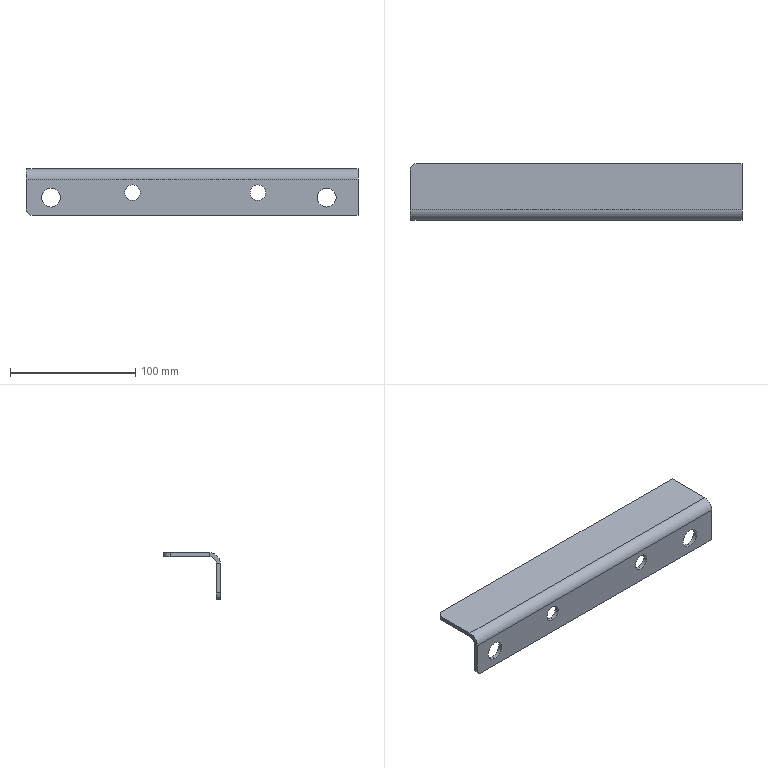Part | SolidWorks | features Fillet 1, FlatPattern 1, ICE 1, SMBaseFlange 1, SheetMetal 1 | 1 solid | 24 faces | box 265 x 45 x 37 mm | volume 62470 mm3 | cylinder 12 | plane 12 | commonest cylinder face diameters 12.5 x4 15 x4 10 x3 16.4 x1
STEP:
#1=CARTESIAN_POINT('',(-112.5,0.,-30.5));
#2=VERTEX_POINT('',#1);
#3=CARTESIAN_POINT('',(-112.5,0.,-15.5));
#4=VERTEX_POINT('',#3);
#5=CARTESIAN_POINT('',(-112.5,0.,-23.));
#6=DIRECTION('',(0.,1.,0.));
#7=DIRECTION('',(0.,0.,1.));
#8=AXIS2_PLACEMENT_3D('',#5,#6,#7);
#9=CIRCLE('',#8,7.5);
#10=EDGE_CURVE('',#2,#4,#9,.T.);
#11=ORIENTED_EDGE('',*,*,#10,.F.);
#12=CARTESIAN_POINT('',(-112.5,3.2,-30.5));
#13=VERTEX_POINT('',#12);
#14=CARTESIAN_POINT('',(-112.5,0.,-30.5));
#15=DIRECTION('',(0.,1.,0.));
#16=VECTOR('',#15,1000.);
#17=LINE('',#14,#16);
#18=EDGE_CURVE('',#2,#13,#17,.T.);
#19=ORIENTED_EDGE('',*,*,#18,.T.);
#20=CARTESIAN_POINT('',(-112.5,3.2,-15.5));
#21=VERTEX_POINT('',#20);
#22=CARTESIAN_POINT('',(-112.5,3.2,-23.));
#23=DIRECTION('',(0.,1.,0.));
#24=DIRECTION('',(0.,0.,1.));
#25=AXIS2_PLACEMENT_3D('',#22,#23,#24);
#26=CIRCLE('',#25,7.5);
#27=EDGE_CURVE('',#13,#21,#26,.T.);
#28=ORIENTED_EDGE('',*,*,#27,.T.);
#29=CARTESIAN_POINT('',(-112.5,0.,-15.5));
#30=DIRECTION('',(0.,1.,0.));
#31=VECTOR('',#30,1000.);
#32=LINE('',#29,#31);
#33=EDGE_CURVE('',#4,#21,#32,.T.);
#34=ORIENTED_EDGE('',*,*,#33,.F.);
#35=EDGE_LOOP('',(#11,#19,#28,#34));
#36=FACE_OUTER_BOUND('',#35,.T.);
#37=CARTESIAN_POINT('',(-112.5,0.,-23.));
#38=DIRECTION('',(0.,1.,0.));
#39=DIRECTION('',(0.,0.,1.));
#40=AXIS2_PLACEMENT_3D('',#37,#38,#39);
#41=CYLINDRICAL_SURFACE('',#40,7.5);
#42=ADVANCED_FACE('',(#36),#41,.F.);
#43=CARTESIAN_POINT('',(107.5,0.,-30.5));
#44=VERTEX_POINT('',#43);
#45=CARTESIAN_POINT('',(107.5,0.,-15.5));
#46=VERTEX_POINT('',#45);
#47=CARTESIAN_POINT('',(107.5,0.,-23.));
#48=DIRECTION('',(0.,1.,0.));
#49=DIRECTION('',(0.,0.,1.));
#50=AXIS2_PLACEMENT_3D('',#47,#48,#49);
#51=CIRCLE('',#50,7.5);
#52=EDGE_CURVE('',#44,#46,#51,.T.);
#53=ORIENTED_EDGE('',*,*,#52,.F.);
#54=CARTESIAN_POINT('',(107.5,3.2,-30.5));
#55=VERTEX_POINT('',#54);
#56=CARTESIAN_POINT('',(107.5,0.,-30.5));
#57=DIRECTION('',(0.,1.,0.));
#58=VECTOR('',#57,1000.);
#59=LINE('',#56,#58);
#60=EDGE_CURVE('',#44,#55,#59,.T.);
#61=ORIENTED_EDGE('',*,*,#60,.T.);
#62=CARTESIAN_POINT('',(107.5,3.2,-15.5));
#63=VERTEX_POINT('',#62);
#64=CARTESIAN_POINT('',(107.5,3.2,-23.));
#65=DIRECTION('',(0.,1.,0.));
#66=DIRECTION('',(0.,0.,1.));
#67=AXIS2_PLACEMENT_3D('',#64,#65,#66);
#68=CIRCLE('',#67,7.5);
#69=EDGE_CURVE('',#55,#63,#68,.T.);
#70=ORIENTED_EDGE('',*,*,#69,.T.);
#71=CARTESIAN_POINT('',(107.5,0.,-15.5));
#72=DIRECTION('',(0.,1.,0.));
#73=VECTOR('',#72,1000.);
#74=LINE('',#71,#73);
#75=EDGE_CURVE('',#46,#63,#74,.T.);
#76=ORIENTED_EDGE('',*,*,#75,.F.);
#77=EDGE_LOOP('',(#53,#61,#70,#76));
#78=FACE_OUTER_BOUND('',#77,.T.);
#79=CARTESIAN_POINT('',(107.5,0.,-23.));
#80=DIRECTION('',(0.,1.,0.));
#81=DIRECTION('',(0.,0.,1.));
#82=AXIS2_PLACEMENT_3D('',#79,#80,#81);
#83=CYLINDRICAL_SURFACE('',#82,7.5);
#84=ADVANCED_FACE('',(#78),#83,.F.);
#85=CARTESIAN_POINT('',(52.5,0.,-25.25));
#86=VERTEX_POINT('',#85);
#87=CARTESIAN_POINT('',(52.5,0.,-12.75));
#88=VERTEX_POINT('',#87);
#89=CARTESIAN_POINT('',(52.5,0.,-19.));
#90=DIRECTION('',(0.,1.,0.));
#91=DIRECTION('',(0.,0.,1.));
#92=AXIS2_PLACEMENT_3D('',#89,#90,#91);
#93=CIRCLE('',#92,6.25);
#94=EDGE_CURVE('',#86,#88,#93,.T.);
#95=ORIENTED_EDGE('',*,*,#94,.F.);
#96=CARTESIAN_POINT('',(52.5,3.2,-25.25));
#97=VERTEX_POINT('',#96);
#98=CARTESIAN_POINT('',(52.5,0.,-25.25));
#99=DIRECTION('',(0.,1.,0.));
#100=VECTOR('',#99,1000.);
#101=LINE('',#98,#100);
#102=EDGE_CURVE('',#86,#97,#101,.T.);
#103=ORIENTED_EDGE('',*,*,#102,.T.);
#104=CARTESIAN_POINT('',(52.5,3.2,-12.75));
#105=VERTEX_POINT('',#104);
#106=CARTESIAN_POINT('',(52.5,3.2,-19.));
#107=DIRECTION('',(0.,1.,0.));
#108=DIRECTION('',(0.,0.,1.));
#109=AXIS2_PLACEMENT_3D('',#106,#107,#108);
#110=CIRCLE('',#109,6.25);
#111=EDGE_CURVE('',#97,#105,#110,.T.);
#112=ORIENTED_EDGE('',*,*,#111,.T.);
#113=CARTESIAN_POINT('',(52.5,0.,-12.75));
#114=DIRECTION('',(0.,1.,0.));
#115=VECTOR('',#114,1000.);
#116=LINE('',#113,#115);
#117=EDGE_CURVE('',#88,#105,#116,.T.);
#118=ORIENTED_EDGE('',*,*,#117,.F.);
#119=EDGE_LOOP('',(#95,#103,#112,#118));
#120=FACE_OUTER_BOUND('',#119,.T.);
#121=CARTESIAN_POINT('',(52.5,0.,-19.));
#122=DIRECTION('',(0.,1.,0.));
#123=DIRECTION('',(0.,0.,1.));
#124=AXIS2_PLACEMENT_3D('',#121,#122,#123);
#125=CYLINDRICAL_SURFACE('',#124,6.25);
#126=ADVANCED_FACE('',(#120),#125,.F.);
#127=CARTESIAN_POINT('',(-47.5,0.,-25.25));
#128=VERTEX_POINT('',#127);
#129=CARTESIAN_POINT('',(-47.5,0.,-12.75));
#130=VERTEX_POINT('',#129);
#131=CARTESIAN_POINT('',(-47.5,0.,-19.));
#132=DIRECTION('',(0.,1.,0.));
#133=DIRECTION('',(0.,0.,1.));
#134=AXIS2_PLACEMENT_3D('',#131,#132,#133);
#135=CIRCLE('',#134,6.25);
#136=EDGE_CURVE('',#128,#130,#135,.T.);
#137=ORIENTED_EDGE('',*,*,#136,.F.);
#138=CARTESIAN_POINT('',(-47.5,3.2,-25.25));
#139=VERTEX_POINT('',#138);
#140=CARTESIAN_POINT('',(-47.5,0.,-25.25));
#141=DIRECTION('',(0.,1.,0.));
#142=VECTOR('',#141,1000.);
#143=LINE('',#140,#142);
#144=EDGE_CURVE('',#128,#139,#143,.T.);
#145=ORIENTED_EDGE('',*,*,#144,.T.);
#146=CARTESIAN_POINT('',(-47.5,3.2,-12.75));
#147=VERTEX_POINT('',#146);
#148=CARTESIAN_POINT('',(-47.5,3.2,-19.));
#149=DIRECTION('',(0.,1.,0.));
#150=DIRECTION('',(0.,0.,1.));
#151=AXIS2_PLACEMENT_3D('',#148,#149,#150);
#152=CIRCLE('',#151,6.25);
#153=EDGE_CURVE('',#139,#147,#152,.T.);
#154=ORIENTED_EDGE('',*,*,#153,.T.);
#155=CARTESIAN_POINT('',(-47.5,0.,-12.75));
#156=DIRECTION('',(0.,1.,0.));
#157=VECTOR('',#156,1000.);
#158=LINE('',#155,#157);
#159=EDGE_CURVE('',#130,#147,#158,.T.);
#160=ORIENTED_EDGE('',*,*,#159,.F.);
#161=EDGE_LOOP('',(#137,#145,#154,#160));
#162=FACE_OUTER_BOUND('',#161,.T.);
#163=CARTESIAN_POINT('',(-47.5,0.,-19.));
#164=DIRECTION('',(0.,1.,0.));
#165=DIRECTION('',(0.,0.,1.));
#166=AXIS2_PLACEMENT_3D('',#163,#164,#165);
#167=CYLINDRICAL_SURFACE('',#166,6.25);
#168=ADVANCED_FACE('',(#162),#167,.F.);
#169=CARTESIAN_POINT('',(132.5,8.2,0.));
#170=VERTEX_POINT('',#169);
#171=CARTESIAN_POINT('',(132.5,8.2,-3.2));
#172=VERTEX_POINT('',#171);
#173=CARTESIAN_POINT('',(132.5,8.2,0.));
#174=DIRECTION('',(0.,0.,-1.));
#175=VECTOR('',#174,1000.);
#176=LINE('',#173,#175);
#177=EDGE_CURVE('',#170,#172,#176,.T.);
#178=ORIENTED_EDGE('',*,*,#177,.F.);
#179=CARTESIAN_POINT('',(132.5,0.,-8.2));
#180=VERTEX_POINT('',#179);
#181=CARTESIAN_POINT('',(132.5,8.2,-8.2));
#182=DIRECTION('',(-1.,0.,0.));
#183=DIRECTION('',(0.,0.,-1.));
#184=AXIS2_PLACEMENT_3D('',#181,#182,#183);
#185=CIRCLE('',#184,8.2);
#186=EDGE_CURVE('',#180,#170,#185,.T.);
#187=ORIENTED_EDGE('',*,*,#186,.F.);
#188=CARTESIAN_POINT('',(132.5,3.2,-8.2));
#189=VERTEX_POINT('',#188);
#190=CARTESIAN_POINT('',(132.5,3.2,-8.2));
#191=DIRECTION('',(0.,-1.,0.));
#192=VECTOR('',#191,1000.);
#193=LINE('',#190,#192);
#194=EDGE_CURVE('',#189,#180,#193,.T.);
#195=ORIENTED_EDGE('',*,*,#194,.F.);
#196=CARTESIAN_POINT('',(132.5,8.2,-8.2));
#197=DIRECTION('',(-1.,0.,0.));
#198=DIRECTION('',(0.,0.,-1.));
#199=AXIS2_PLACEMENT_3D('',#196,#197,#198);
#200=CIRCLE('',#199,5.);
#201=EDGE_CURVE('',#189,#172,#200,.T.);
#202=ORIENTED_EDGE('',*,*,#201,.T.);
#203=EDGE_LOOP('',(#178,#187,#195,#202));
#204=FACE_OUTER_BOUND('',#203,.T.);
#205=CARTESIAN_POINT('',(132.5,8.2,0.));
#206=DIRECTION('',(1.,0.,0.));
#207=DIRECTION('',(0.,0.,-1.));
#208=AXIS2_PLACEMENT_3D('',#205,#206,#207);
#209=PLANE('',#208);
#210=ADVANCED_FACE('',(#204),#209,.T.);
#211=CARTESIAN_POINT('',(132.5,45.,0.));
#212=VERTEX_POINT('',#211);
#213=CARTESIAN_POINT('',(132.5,0.,0.));
#214=DIRECTION('',(0.,1.,0.));
#215=VECTOR('',#214,1000.);
#216=LINE('',#213,#215);
#217=EDGE_CURVE('',#170,#212,#216,.T.);
#218=ORIENTED_EDGE('',*,*,#217,.F.);
#219=ORIENTED_EDGE('',*,*,#177,.T.);
#220=CARTESIAN_POINT('',(132.5,45.,-3.2));
#221=VERTEX_POINT('',#220);
#222=CARTESIAN_POINT('',(132.5,0.,-3.2));
#223=DIRECTION('',(0.,1.,0.));
#224=VECTOR('',#223,1000.);
#225=LINE('',#222,#224);
#226=EDGE_CURVE('',#172,#221,#225,.T.);
#227=ORIENTED_EDGE('',*,*,#226,.T.);
#228=CARTESIAN_POINT('',(132.5,45.,0.));
#229=DIRECTION('',(0.,0.,-1.));
#230=VECTOR('',#229,1000.);
#231=LINE('',#228,#230);
#232=EDGE_CURVE('',#212,#221,#231,.T.);
#233=ORIENTED_EDGE('',*,*,#232,.F.);
#234=EDGE_LOOP('',(#218,#219,#227,#233));
#235=FACE_OUTER_BOUND('',#234,.T.);
#236=CARTESIAN_POINT('',(132.5,3.2,-8.2));
#237=DIRECTION('',(1.,0.,0.));
#238=DIRECTION('',(0.,0.,-1.));
#239=AXIS2_PLACEMENT_3D('',#236,#237,#238);
#240=PLANE('',#239);
#241=ADVANCED_FACE('',(#235),#240,.T.);
#242=CARTESIAN_POINT('',(-132.5,0.,-8.2));
#243=VERTEX_POINT('',#242);
#244=CARTESIAN_POINT('',(-132.5,3.2,-8.2));
#245=VERTEX_POINT('',#244);
#246=CARTESIAN_POINT('',(-132.5,0.,-8.2));
#247=DIRECTION('',(0.,1.,0.));
#248=VECTOR('',#247,1000.);
#249=LINE('',#246,#248);
#250=EDGE_CURVE('',#243,#245,#249,.T.);
#251=ORIENTED_EDGE('',*,*,#250,.F.);
#252=CARTESIAN_POINT('',(-132.5,8.2,0.));
#253=VERTEX_POINT('',#252);
#254=CARTESIAN_POINT('',(-132.5,8.2,-8.2));
#255=DIRECTION('',(-1.,0.,0.));
#256=DIRECTION('',(0.,0.,-1.));
#257=AXIS2_PLACEMENT_3D('',#254,#255,#256);
#258=CIRCLE('',#257,8.2);
#259=EDGE_CURVE('',#243,#253,#258,.T.);
#260=ORIENTED_EDGE('',*,*,#259,.T.);
#261=CARTESIAN_POINT('',(-132.5,8.2,-3.2));
#262=VERTEX_POINT('',#261);
#263=CARTESIAN_POINT('',(-132.5,8.2,-3.2));
#264=DIRECTION('',(0.,0.,1.));
#265=VECTOR('',#264,1000.);
#266=LINE('',#263,#265);
#267=EDGE_CURVE('',#262,#253,#266,.T.);
#268=ORIENTED_EDGE('',*,*,#267,.F.);
#269=CARTESIAN_POINT('',(-132.5,8.2,-8.2));
#270=DIRECTION('',(-1.,0.,0.));
#271=DIRECTION('',(0.,0.,-1.));
#272=AXIS2_PLACEMENT_3D('',#269,#270,#271);
#273=CIRCLE('',#272,5.);
#274=EDGE_CURVE('',#245,#262,#273,.T.);
#275=ORIENTED_EDGE('',*,*,#274,.F.);
#276=EDGE_LOOP('',(#251,#260,#268,#275));
#277=FACE_OUTER_BOUND('',#276,.T.);
#278=CARTESIAN_POINT('',(-132.5,0.,-8.2));
#279=DIRECTION('',(-1.,0.,0.));
#280=DIRECTION('',(0.,0.,1.));
#281=AXIS2_PLACEMENT_3D('',#278,#279,#280);
#282=PLANE('',#281);
#283=ADVANCED_FACE('',(#277),#282,.T.);
#284=CARTESIAN_POINT('',(-132.5,3.2,-32.));
#285=VERTEX_POINT('',#284);
#286=CARTESIAN_POINT('',(-132.5,3.2,0.));
#287=DIRECTION('',(0.,0.,1.));
#288=VECTOR('',#287,1000.);
#289=LINE('',#286,#288);
#290=EDGE_CURVE('',#285,#245,#289,.T.);
#291=ORIENTED_EDGE('',*,*,#290,.F.);
#292=CARTESIAN_POINT('',(-132.5,0.,-32.));
#293=VERTEX_POINT('',#292);
#294=CARTESIAN_POINT('',(-132.5,8.2,-32.));
#295=DIRECTION('',(0.,-1.,0.));
#296=VECTOR('',#295,1000.);
#297=LINE('',#294,#296);
#298=EDGE_CURVE('',#285,#293,#297,.T.);
#299=ORIENTED_EDGE('',*,*,#298,.T.);
#300=CARTESIAN_POINT('',(-132.5,0.,0.));
#301=DIRECTION('',(0.,0.,1.));
#302=VECTOR('',#301,1000.);
#303=LINE('',#300,#302);
#304=EDGE_CURVE('',#293,#243,#303,.T.);
#305=ORIENTED_EDGE('',*,*,#304,.T.);
#306=ORIENTED_EDGE('',*,*,#250,.T.);
#307=EDGE_LOOP('',(#291,#299,#305,#306));
#308=FACE_OUTER_BOUND('',#307,.T.);
#309=CARTESIAN_POINT('',(-132.5,8.2,-3.2));
#310=DIRECTION('',(-1.,0.,0.));
#311=DIRECTION('',(0.,0.,1.));
#312=AXIS2_PLACEMENT_3D('',#309,#310,#311);
#313=PLANE('',#312);
#314=ADVANCED_FACE('',(#308),#313,.T.);
#315=CARTESIAN_POINT('',(-132.5,40.,-3.2));
#316=VERTEX_POINT('',#315);
#317=CARTESIAN_POINT('',(-132.5,0.,-3.2));
#318=DIRECTION('',(0.,1.,0.));
#319=VECTOR('',#318,1000.);
#320=LINE('',#317,#319);
#321=EDGE_CURVE('',#262,#316,#320,.T.);
#322=ORIENTED_EDGE('',*,*,#321,.T.);
#323=CARTESIAN_POINT('',(-127.5,45.,-3.2));
#324=VERTEX_POINT('',#323);
#325=CARTESIAN_POINT('',(-127.5,40.,-3.2));
#326=DIRECTION('',(0.,0.,-1.));
#327=DIRECTION('',(1.,0.,0.));
#328=AXIS2_PLACEMENT_3D('',#325,#326,#327);
#329=CIRCLE('',#328,5.);
#330=EDGE_CURVE('',#316,#324,#329,.T.);
#331=ORIENTED_EDGE('',*,*,#330,.T.);
#332=CARTESIAN_POINT('',(132.5,45.,-3.2));
#333=DIRECTION('',(-1.,0.,0.));
#334=VECTOR('',#333,1000.);
#335=LINE('',#332,#334);
#336=EDGE_CURVE('',#221,#324,#335,.T.);
#337=ORIENTED_EDGE('',*,*,#336,.F.);
#338=ORIENTED_EDGE('',*,*,#226,.F.);
#339=CARTESIAN_POINT('',(132.5,8.2,-3.2));
#340=DIRECTION('',(-1.,0.,0.));
#341=VECTOR('',#340,1000.);
#342=LINE('',#339,#341);
#343=EDGE_CURVE('',#172,#262,#342,.T.);
#344=ORIENTED_EDGE('',*,*,#343,.T.);
#345=EDGE_LOOP('',(#322,#331,#337,#338,#344));
#346=FACE_OUTER_BOUND('',#345,.T.);
#347=CARTESIAN_POINT('',(132.5,0.,-3.2));
#348=DIRECTION('',(0.,0.,1.));
#349=DIRECTION('',(1.,0.,0.));
#350=AXIS2_PLACEMENT_3D('',#347,#348,#349);
#351=PLANE('',#350);
#352=ADVANCED_FACE('',(#346),#351,.F.);
#353=ORIENTED_EDGE('',*,*,#336,.T.);
#354=CARTESIAN_POINT('',(-127.5,45.,0.));
#355=VERTEX_POINT('',#354);
#356=CARTESIAN_POINT('',(-127.5,45.,0.));
#357=DIRECTION('',(0.,0.,1.));
#358=VECTOR('',#357,1000.);
#359=LINE('',#356,#358);
#360=EDGE_CURVE('',#324,#355,#359,.T.);
#361=ORIENTED_EDGE('',*,*,#360,.T.);
#362=CARTESIAN_POINT('',(132.5,45.,0.));
#363=DIRECTION('',(-1.,0.,0.));
#364=VECTOR('',#363,1000.);
#365=LINE('',#362,#364);
#366=EDGE_CURVE('',#212,#355,#365,.T.);
#367=ORIENTED_EDGE('',*,*,#366,.F.);
#368=ORIENTED_EDGE('',*,*,#232,.T.);
#369=EDGE_LOOP('',(#353,#361,#367,#368));
#370=FACE_OUTER_BOUND('',#369,.T.);
#371=CARTESIAN_POINT('',(132.5,45.,0.));
#372=DIRECTION('',(0.,1.,0.));
#373=DIRECTION('',(0.,0.,1.));
#374=AXIS2_PLACEMENT_3D('',#371,#372,#373);
#375=PLANE('',#374);
#376=ADVANCED_FACE('',(#370),#375,.T.);
#377=ORIENTED_EDGE('',*,*,#366,.T.);
#378=CARTESIAN_POINT('',(-132.5,40.,0.));
#379=VERTEX_POINT('',#378);
#380=CARTESIAN_POINT('',(-127.5,40.,0.));
#381=DIRECTION('',(0.,0.,1.));
#382=DIRECTION('',(1.,0.,0.));
#383=AXIS2_PLACEMENT_3D('',#380,#381,#382);
#384=CIRCLE('',#383,5.);
#385=EDGE_CURVE('',#355,#379,#384,.T.);
#386=ORIENTED_EDGE('',*,*,#385,.T.);
#387=CARTESIAN_POINT('',(-132.5,0.,0.));
#388=DIRECTION('',(0.,1.,0.));
#389=VECTOR('',#388,1000.);
#390=LINE('',#387,#389);
#391=EDGE_CURVE('',#253,#379,#390,.T.);
#392=ORIENTED_EDGE('',*,*,#391,.F.);
#393=CARTESIAN_POINT('',(132.5,8.2,0.));
#394=DIRECTION('',(-1.,0.,0.));
#395=VECTOR('',#394,1000.);
#396=LINE('',#393,#395);
#397=EDGE_CURVE('',#170,#253,#396,.T.);
#398=ORIENTED_EDGE('',*,*,#397,.F.);
#399=ORIENTED_EDGE('',*,*,#217,.T.);
#400=EDGE_LOOP('',(#377,#386,#392,#398,#399));
#401=FACE_OUTER_BOUND('',#400,.T.);
#402=CARTESIAN_POINT('',(132.5,0.,0.));
#403=DIRECTION('',(0.,0.,1.));
#404=DIRECTION('',(1.,0.,0.));
#405=AXIS2_PLACEMENT_3D('',#402,#403,#404);
#406=PLANE('',#405);
#407=ADVANCED_FACE('',(#401),#406,.T.);
#408=ORIENTED_EDGE('',*,*,#259,.F.);
#409=CARTESIAN_POINT('',(132.5,0.,-8.2));
#410=DIRECTION('',(-1.,0.,0.));
#411=VECTOR('',#410,1000.);
#412=LINE('',#409,#411);
#413=EDGE_CURVE('',#180,#243,#412,.T.);
#414=ORIENTED_EDGE('',*,*,#413,.F.);
#415=ORIENTED_EDGE('',*,*,#186,.T.);
#416=ORIENTED_EDGE('',*,*,#397,.T.);
#417=EDGE_LOOP('',(#408,#414,#415,#416));
#418=FACE_OUTER_BOUND('',#417,.T.);
#419=CARTESIAN_POINT('',(132.5,8.2,-8.2));
#420=DIRECTION('',(-1.,0.,0.));
#421=DIRECTION('',(0.,0.,1.));
#422=AXIS2_PLACEMENT_3D('',#419,#420,#421);
#423=CYLINDRICAL_SURFACE('',#422,8.2);
#424=ADVANCED_FACE('',(#418),#423,.T.);
#425=CARTESIAN_POINT('',(-112.5,0.,-23.));
#426=DIRECTION('',(0.,1.,0.));
#427=DIRECTION('',(0.,0.,1.));
#428=AXIS2_PLACEMENT_3D('',#425,#426,#427);
#429=CIRCLE('',#428,7.5);
#430=EDGE_CURVE('',#4,#2,#429,.T.);
#431=ORIENTED_EDGE('',*,*,#430,.T.);
#432=ORIENTED_EDGE('',*,*,#10,.T.);
#433=EDGE_LOOP('',(#431,#432));
#434=FACE_BOUND('',#433,.T.);
#435=CARTESIAN_POINT('',(107.5,0.,-23.));
#436=DIRECTION('',(0.,1.,0.));
#437=DIRECTION('',(0.,0.,1.));
#438=AXIS2_PLACEMENT_3D('',#435,#436,#437);
#439=CIRCLE('',#438,7.5);
#440=EDGE_CURVE('',#46,#44,#439,.T.);
#441=ORIENTED_EDGE('',*,*,#440,.T.);
#442=ORIENTED_EDGE('',*,*,#52,.T.);
#443=EDGE_LOOP('',(#441,#442));
#444=FACE_BOUND('',#443,.T.);
#445=CARTESIAN_POINT('',(52.5,0.,-19.));
#446=DIRECTION('',(0.,1.,0.));
#447=DIRECTION('',(0.,0.,1.));
#448=AXIS2_PLACEMENT_3D('',#445,#446,#447);
#449=CIRCLE('',#448,6.25);
#450=EDGE_CURVE('',#88,#86,#449,.T.);
#451=ORIENTED_EDGE('',*,*,#450,.T.);
#452=ORIENTED_EDGE('',*,*,#94,.T.);
#453=EDGE_LOOP('',(#451,#452));
#454=FACE_BOUND('',#453,.T.);
#455=CARTESIAN_POINT('',(-47.5,0.,-19.));
#456=DIRECTION('',(0.,1.,0.));
#457=DIRECTION('',(0.,0.,1.));
#458=AXIS2_PLACEMENT_3D('',#455,#456,#457);
#459=CIRCLE('',#458,6.25);
#460=EDGE_CURVE('',#130,#128,#459,.T.);
#461=ORIENTED_EDGE('',*,*,#460,.T.);
#462=ORIENTED_EDGE('',*,*,#136,.T.);
#463=EDGE_LOOP('',(#461,#462));
#464=FACE_BOUND('',#463,.T.);
#465=ORIENTED_EDGE('',*,*,#304,.F.);
#466=CARTESIAN_POINT('',(-127.5,0.,-37.));
#467=VERTEX_POINT('',#466);
#468=CARTESIAN_POINT('',(-127.5,0.,-32.));
#469=DIRECTION('',(0.,-1.,0.));
#470=DIRECTION('',(0.,0.,-1.));
#471=AXIS2_PLACEMENT_3D('',#468,#469,#470);
#472=CIRCLE('',#471,5.);
#473=EDGE_CURVE('',#293,#467,#472,.T.);
#474=ORIENTED_EDGE('',*,*,#473,.T.);
#475=CARTESIAN_POINT('',(132.5,0.,-37.));
#476=VERTEX_POINT('',#475);
#477=CARTESIAN_POINT('',(132.5,0.,-37.));
#478=DIRECTION('',(-1.,0.,0.));
#479=VECTOR('',#478,1000.);
#480=LINE('',#477,#479);
#481=EDGE_CURVE('',#476,#467,#480,.T.);
#482=ORIENTED_EDGE('',*,*,#481,.F.);
#483=CARTESIAN_POINT('',(132.5,0.,0.));
#484=DIRECTION('',(0.,0.,1.));
#485=VECTOR('',#484,1000.);
#486=LINE('',#483,#485);
#487=EDGE_CURVE('',#476,#180,#486,.T.);
#488=ORIENTED_EDGE('',*,*,#487,.T.);
#489=ORIENTED_EDGE('',*,*,#413,.T.);
#490=EDGE_LOOP('',(#465,#474,#482,#488,#489));
#491=FACE_OUTER_BOUND('',#490,.T.);
#492=CARTESIAN_POINT('',(132.5,0.,0.));
#493=DIRECTION('',(0.,-1.,0.));
#494=DIRECTION('',(0.,0.,-1.));
#495=AXIS2_PLACEMENT_3D('',#492,#493,#494);
#496=PLANE('',#495);
#497=ADVANCED_FACE('',(#434,#444,#454,#464,#491),#496,.T.);
#498=ORIENTED_EDGE('',*,*,#481,.T.);
#499=CARTESIAN_POINT('',(-127.5,3.2,-37.));
#500=VERTEX_POINT('',#499);
#501=CARTESIAN_POINT('',(-127.5,3.2,-37.));
#502=DIRECTION('',(0.,1.,0.));
#503=VECTOR('',#502,1000.);
#504=LINE('',#501,#503);
#505=EDGE_CURVE('',#467,#500,#504,.T.);
#506=ORIENTED_EDGE('',*,*,#505,.T.);
#507=CARTESIAN_POINT('',(132.5,3.2,-37.));
#508=VERTEX_POINT('',#507);
#509=CARTESIAN_POINT('',(132.5,3.2,-37.));
#510=DIRECTION('',(-1.,0.,0.));
#511=VECTOR('',#510,1000.);
#512=LINE('',#509,#511);
#513=EDGE_CURVE('',#508,#500,#512,.T.);
#514=ORIENTED_EDGE('',*,*,#513,.F.);
#515=CARTESIAN_POINT('',(132.5,3.2,-37.));
#516=DIRECTION('',(0.,-1.,0.));
#517=VECTOR('',#516,1000.);
#518=LINE('',#515,#517);
#519=EDGE_CURVE('',#508,#476,#518,.T.);
#520=ORIENTED_EDGE('',*,*,#519,.T.);
#521=EDGE_LOOP('',(#498,#506,#514,#520));
#522=FACE_OUTER_BOUND('',#521,.T.);
#523=CARTESIAN_POINT('',(132.5,3.2,-37.));
#524=DIRECTION('',(0.,0.,-1.));
#525=DIRECTION('',(-1.,0.,0.));
#526=AXIS2_PLACEMENT_3D('',#523,#524,#525);
#527=PLANE('',#526);
#528=ADVANCED_FACE('',(#522),#527,.T.);
#529=CARTESIAN_POINT('',(-112.5,3.2,-23.));
#530=DIRECTION('',(0.,1.,0.));
#531=DIRECTION('',(0.,0.,1.));
#532=AXIS2_PLACEMENT_3D('',#529,#530,#531);
#533=CIRCLE('',#532,7.5);
#534=EDGE_CURVE('',#21,#13,#533,.T.);
#535=ORIENTED_EDGE('',*,*,#534,.F.);
#536=ORIENTED_EDGE('',*,*,#27,.F.);
#537=EDGE_LOOP('',(#535,#536));
#538=FACE_BOUND('',#537,.T.);
#539=CARTESIAN_POINT('',(107.5,3.2,-23.));
#540=DIRECTION('',(0.,1.,0.));
#541=DIRECTION('',(0.,0.,1.));
#542=AXIS2_PLACEMENT_3D('',#539,#540,#541);
#543=CIRCLE('',#542,7.5);
#544=EDGE_CURVE('',#63,#55,#543,.T.);
#545=ORIENTED_EDGE('',*,*,#544,.F.);
#546=ORIENTED_EDGE('',*,*,#69,.F.);
#547=EDGE_LOOP('',(#545,#546));
#548=FACE_BOUND('',#547,.T.);
#549=CARTESIAN_POINT('',(52.5,3.2,-19.));
#550=DIRECTION('',(0.,1.,0.));
#551=DIRECTION('',(0.,0.,1.));
#552=AXIS2_PLACEMENT_3D('',#549,#550,#551);
#553=CIRCLE('',#552,6.25);
#554=EDGE_CURVE('',#105,#97,#553,.T.);
#555=ORIENTED_EDGE('',*,*,#554,.F.);
#556=ORIENTED_EDGE('',*,*,#111,.F.);
#557=EDGE_LOOP('',(#555,#556));
#558=FACE_BOUND('',#557,.T.);
#559=CARTESIAN_POINT('',(-47.5,3.2,-19.));
#560=DIRECTION('',(0.,1.,0.));
#561=DIRECTION('',(0.,0.,1.));
#562=AXIS2_PLACEMENT_3D('',#559,#560,#561);
#563=CIRCLE('',#562,6.25);
#564=EDGE_CURVE('',#147,#139,#563,.T.);
#565=ORIENTED_EDGE('',*,*,#564,.F.);
#566=ORIENTED_EDGE('',*,*,#153,.F.);
#567=EDGE_LOOP('',(#565,#566));
#568=FACE_BOUND('',#567,.T.);
#569=ORIENTED_EDGE('',*,*,#513,.T.);
#570=CARTESIAN_POINT('',(-127.5,3.2,-32.));
#571=DIRECTION('',(0.,1.,0.));
#572=DIRECTION('',(0.,0.,-1.));
#573=AXIS2_PLACEMENT_3D('',#570,#571,#572);
#574=CIRCLE('',#573,5.);
#575=EDGE_CURVE('',#500,#285,#574,.T.);
#576=ORIENTED_EDGE('',*,*,#575,.T.);
#577=ORIENTED_EDGE('',*,*,#290,.T.);
#578=CARTESIAN_POINT('',(132.5,3.2,-8.2));
#579=DIRECTION('',(-1.,0.,0.));
#580=VECTOR('',#579,1000.);
#581=LINE('',#578,#580);
#582=EDGE_CURVE('',#189,#245,#581,.T.);
#583=ORIENTED_EDGE('',*,*,#582,.F.);
#584=CARTESIAN_POINT('',(132.5,3.2,0.));
#585=DIRECTION('',(0.,0.,1.));
#586=VECTOR('',#585,1000.);
#587=LINE('',#584,#586);
#588=EDGE_CURVE('',#508,#189,#587,.T.);
#589=ORIENTED_EDGE('',*,*,#588,.F.);
#590=EDGE_LOOP('',(#569,#576,#577,#583,#589));
#591=FACE_OUTER_BOUND('',#590,.T.);
#592=CARTESIAN_POINT('',(132.5,3.2,0.));
#593=DIRECTION('',(0.,-1.,0.));
#594=DIRECTION('',(0.,0.,-1.));
#595=AXIS2_PLACEMENT_3D('',#592,#593,#594);
#596=PLANE('',#595);
#597=ADVANCED_FACE('',(#538,#548,#558,#568,#591),#596,.F.);
#598=ORIENTED_EDGE('',*,*,#274,.T.);
#599=ORIENTED_EDGE('',*,*,#343,.F.);
#600=ORIENTED_EDGE('',*,*,#201,.F.);
#601=ORIENTED_EDGE('',*,*,#582,.T.);
#602=EDGE_LOOP('',(#598,#599,#600,#601));
#603=FACE_OUTER_BOUND('',#602,.T.);
#604=CARTESIAN_POINT('',(132.5,8.2,-8.2));
#605=DIRECTION('',(-1.,0.,0.));
#606=DIRECTION('',(0.,0.,1.));
#607=AXIS2_PLACEMENT_3D('',#604,#605,#606);
#608=CYLINDRICAL_SURFACE('',#607,5.);
#609=ADVANCED_FACE('',(#603),#608,.F.);
#610=ORIENTED_EDGE('',*,*,#588,.T.);
#611=ORIENTED_EDGE('',*,*,#194,.T.);
#612=ORIENTED_EDGE('',*,*,#487,.F.);
#613=ORIENTED_EDGE('',*,*,#519,.F.);
#614=EDGE_LOOP('',(#610,#611,#612,#613));
#615=FACE_OUTER_BOUND('',#614,.T.);
#616=CARTESIAN_POINT('',(132.5,8.2,-8.2));
#617=DIRECTION('',(1.,0.,0.));
#618=DIRECTION('',(0.,0.,-1.));
#619=AXIS2_PLACEMENT_3D('',#616,#617,#618);
#620=PLANE('',#619);
#621=ADVANCED_FACE('',(#615),#620,.T.);
#622=ORIENTED_EDGE('',*,*,#391,.T.);
#623=CARTESIAN_POINT('',(-132.5,40.,-3.2));
#624=DIRECTION('',(0.,0.,-1.));
#625=VECTOR('',#624,1000.);
#626=LINE('',#623,#625);
#627=EDGE_CURVE('',#379,#316,#626,.T.);
#628=ORIENTED_EDGE('',*,*,#627,.T.);
#629=ORIENTED_EDGE('',*,*,#321,.F.);
#630=ORIENTED_EDGE('',*,*,#267,.T.);
#631=EDGE_LOOP('',(#622,#628,#629,#630));
#632=FACE_OUTER_BOUND('',#631,.T.);
#633=CARTESIAN_POINT('',(-132.5,8.2,-8.2));
#634=DIRECTION('',(1.,0.,0.));
#635=DIRECTION('',(0.,0.,-1.));
#636=AXIS2_PLACEMENT_3D('',#633,#634,#635);
#637=PLANE('',#636);
#638=ADVANCED_FACE('',(#632),#637,.F.);
#639=ORIENTED_EDGE('',*,*,#144,.F.);
#640=ORIENTED_EDGE('',*,*,#460,.F.);
#641=ORIENTED_EDGE('',*,*,#159,.T.);
#642=ORIENTED_EDGE('',*,*,#564,.T.);
#643=EDGE_LOOP('',(#639,#640,#641,#642));
#644=FACE_OUTER_BOUND('',#643,.T.);
#645=CARTESIAN_POINT('',(-47.5,0.,-19.));
#646=DIRECTION('',(0.,1.,0.));
#647=DIRECTION('',(0.,0.,1.));
#648=AXIS2_PLACEMENT_3D('',#645,#646,#647);
#649=CYLINDRICAL_SURFACE('',#648,6.25);
#650=ADVANCED_FACE('',(#644),#649,.F.);
#651=ORIENTED_EDGE('',*,*,#102,.F.);
#652=ORIENTED_EDGE('',*,*,#450,.F.);
#653=ORIENTED_EDGE('',*,*,#117,.T.);
#654=ORIENTED_EDGE('',*,*,#554,.T.);
#655=EDGE_LOOP('',(#651,#652,#653,#654));
#656=FACE_OUTER_BOUND('',#655,.T.);
#657=CARTESIAN_POINT('',(52.5,0.,-19.));
#658=DIRECTION('',(0.,1.,0.));
#659=DIRECTION('',(0.,0.,1.));
#660=AXIS2_PLACEMENT_3D('',#657,#658,#659);
#661=CYLINDRICAL_SURFACE('',#660,6.25);
#662=ADVANCED_FACE('',(#656),#661,.F.);
#663=ORIENTED_EDGE('',*,*,#60,.F.);
#664=ORIENTED_EDGE('',*,*,#440,.F.);
#665=ORIENTED_EDGE('',*,*,#75,.T.);
#666=ORIENTED_EDGE('',*,*,#544,.T.);
#667=EDGE_LOOP('',(#663,#664,#665,#666));
#668=FACE_OUTER_BOUND('',#667,.T.);
#669=CARTESIAN_POINT('',(107.5,0.,-23.));
#670=DIRECTION('',(0.,1.,0.));
#671=DIRECTION('',(0.,0.,1.));
#672=AXIS2_PLACEMENT_3D('',#669,#670,#671);
#673=CYLINDRICAL_SURFACE('',#672,7.5);
#674=ADVANCED_FACE('',(#668),#673,.F.);
#675=ORIENTED_EDGE('',*,*,#18,.F.);
#676=ORIENTED_EDGE('',*,*,#430,.F.);
#677=ORIENTED_EDGE('',*,*,#33,.T.);
#678=ORIENTED_EDGE('',*,*,#534,.T.);
#679=EDGE_LOOP('',(#675,#676,#677,#678));
#680=FACE_OUTER_BOUND('',#679,.T.);
#681=CARTESIAN_POINT('',(-112.5,0.,-23.));
#682=DIRECTION('',(0.,1.,0.));
#683=DIRECTION('',(0.,0.,1.));
#684=AXIS2_PLACEMENT_3D('',#681,#682,#683);
#685=CYLINDRICAL_SURFACE('',#684,7.5);
#686=ADVANCED_FACE('',(#680),#685,.F.);
#687=ORIENTED_EDGE('',*,*,#385,.F.);
#688=ORIENTED_EDGE('',*,*,#360,.F.);
#689=ORIENTED_EDGE('',*,*,#330,.F.);
#690=ORIENTED_EDGE('',*,*,#627,.F.);
#691=EDGE_LOOP('',(#687,#688,#689,#690));
#692=FACE_OUTER_BOUND('',#691,.T.);
#693=CARTESIAN_POINT('',(-127.5,40.,-8.2));
#694=DIRECTION('',(0.,0.,1.));
#695=DIRECTION('',(0.,-1.,0.));
#696=AXIS2_PLACEMENT_3D('',#693,#694,#695);
#697=CYLINDRICAL_SURFACE('',#696,5.);
#698=ADVANCED_FACE('',(#692),#697,.T.);
#699=ORIENTED_EDGE('',*,*,#575,.F.);
#700=ORIENTED_EDGE('',*,*,#505,.F.);
#701=ORIENTED_EDGE('',*,*,#473,.F.);
#702=ORIENTED_EDGE('',*,*,#298,.F.);
#703=EDGE_LOOP('',(#699,#700,#701,#702));
#704=FACE_OUTER_BOUND('',#703,.T.);
#705=CARTESIAN_POINT('',(-127.5,8.2,-32.));
#706=DIRECTION('',(0.,-1.,0.));
#707=DIRECTION('',(0.,0.,-1.));
#708=AXIS2_PLACEMENT_3D('',#705,#706,#707);
#709=CYLINDRICAL_SURFACE('',#708,5.);
#710=ADVANCED_FACE('',(#704),#709,.T.);
#711=CLOSED_SHELL('',(#42,#84,#126,#168,#210,#241,#283,#314,#352,#376,#407,#424,#497,#528,#597,#609,#621,#638,#650,#662,#674,#686,#698,#710));
#712=MANIFOLD_SOLID_BREP('',#711);
#713=CARTESIAN_POINT('',(0.,0.,0.));
#714=DIRECTION('',(0.,0.,1.));
#715=DIRECTION('',(1.,0.,0.));
#716=AXIS2_PLACEMENT_3D('',#713,#714,#715);
#717=(LENGTH_UNIT()NAMED_UNIT(*)SI_UNIT(.MILLI.,.METRE.));
#718=UNCERTAINTY_MEASURE_WITH_UNIT(LENGTH_MEASURE(0.00001),#717,'','');
#719=(NAMED_UNIT(*)PLANE_ANGLE_UNIT()SI_UNIT($,.RADIAN.));
#720=(NAMED_UNIT(*)SI_UNIT($,.STERADIAN.)SOLID_ANGLE_UNIT());
#721=(GEOMETRIC_REPRESENTATION_CONTEXT(3)GLOBAL_UNCERTAINTY_ASSIGNED_CONTEXT((#718))GLOBAL_UNIT_ASSIGNED_CONTEXT((#717,#719,#720))REPRESENTATION_CONTEXT('',''));
#722=ADVANCED_BREP_SHAPE_REPRESENTATION('',(#712,#716),#721);